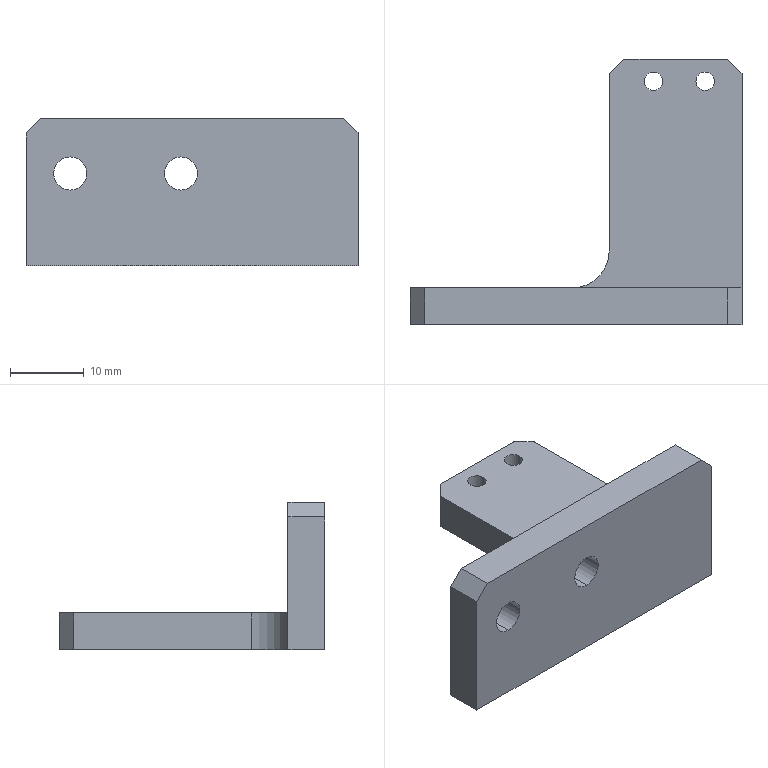Part | STEP file | 10-10 sensor fixing block | 1 solid | 22 faces | box 45 x 36 x 20 mm | volume 7069 mm3 | plane 13 | cylinder 9 | commonest cylinder face diameters 2.5 x4 4.5 x4 10 x1
STEP:
#1=CARTESIAN_POINT('',(34.25,33.,5.));
#2=VERTEX_POINT('',#1);
#3=CARTESIAN_POINT('',(31.75,33.,5.));
#4=VERTEX_POINT('',#3);
#5=CARTESIAN_POINT('',(33.,33.,5.));
#6=DIRECTION('',(0.,0.,-1.));
#7=DIRECTION('',(0.,1.,0.));
#8=AXIS2_PLACEMENT_3D('',#5,#6,#7);
#9=CIRCLE('',#8,1.25);
#10=EDGE_CURVE('',#2,#4,#9,.T.);
#11=ORIENTED_EDGE('',*,*,#10,.F.);
#12=CARTESIAN_POINT('',(34.25,33.,0.));
#13=VERTEX_POINT('',#12);
#14=CARTESIAN_POINT('',(34.25,33.,0.));
#15=DIRECTION('',(0.,0.,-1.));
#16=VECTOR('',#15,1000.);
#17=LINE('',#14,#16);
#18=EDGE_CURVE('',#2,#13,#17,.T.);
#19=ORIENTED_EDGE('',*,*,#18,.T.);
#20=CARTESIAN_POINT('',(31.75,33.,0.));
#21=VERTEX_POINT('',#20);
#22=CARTESIAN_POINT('',(33.,33.,0.));
#23=DIRECTION('',(0.,0.,-1.));
#24=DIRECTION('',(-1.,0.,0.));
#25=AXIS2_PLACEMENT_3D('',#22,#23,#24);
#26=CIRCLE('',#25,1.25);
#27=EDGE_CURVE('',#13,#21,#26,.T.);
#28=ORIENTED_EDGE('',*,*,#27,.T.);
#29=CARTESIAN_POINT('',(31.75,33.,0.));
#30=DIRECTION('',(0.,0.,-1.));
#31=VECTOR('',#30,1000.);
#32=LINE('',#29,#31);
#33=EDGE_CURVE('',#4,#21,#32,.T.);
#34=ORIENTED_EDGE('',*,*,#33,.F.);
#35=EDGE_LOOP('',(#11,#19,#28,#34));
#36=FACE_OUTER_BOUND('',#35,.T.);
#37=CARTESIAN_POINT('',(33.,33.,0.));
#38=DIRECTION('',(0.,0.,-1.));
#39=DIRECTION('',(-1.,0.,0.));
#40=AXIS2_PLACEMENT_3D('',#37,#38,#39);
#41=CYLINDRICAL_SURFACE('',#40,1.25);
#42=ADVANCED_FACE('',(#36),#41,.F.);
#43=CARTESIAN_POINT('',(41.25,33.,5.));
#44=VERTEX_POINT('',#43);
#45=CARTESIAN_POINT('',(38.75,33.,5.));
#46=VERTEX_POINT('',#45);
#47=CARTESIAN_POINT('',(40.,33.,5.));
#48=DIRECTION('',(0.,0.,-1.));
#49=DIRECTION('',(0.,1.,0.));
#50=AXIS2_PLACEMENT_3D('',#47,#48,#49);
#51=CIRCLE('',#50,1.25);
#52=EDGE_CURVE('',#44,#46,#51,.T.);
#53=ORIENTED_EDGE('',*,*,#52,.F.);
#54=CARTESIAN_POINT('',(41.25,33.,0.));
#55=VERTEX_POINT('',#54);
#56=CARTESIAN_POINT('',(41.25,33.,0.));
#57=DIRECTION('',(0.,0.,-1.));
#58=VECTOR('',#57,1000.);
#59=LINE('',#56,#58);
#60=EDGE_CURVE('',#44,#55,#59,.T.);
#61=ORIENTED_EDGE('',*,*,#60,.T.);
#62=CARTESIAN_POINT('',(38.75,33.,0.));
#63=VERTEX_POINT('',#62);
#64=CARTESIAN_POINT('',(40.,33.,0.));
#65=DIRECTION('',(0.,0.,-1.));
#66=DIRECTION('',(-1.,0.,0.));
#67=AXIS2_PLACEMENT_3D('',#64,#65,#66);
#68=CIRCLE('',#67,1.25);
#69=EDGE_CURVE('',#55,#63,#68,.T.);
#70=ORIENTED_EDGE('',*,*,#69,.T.);
#71=CARTESIAN_POINT('',(38.75,33.,0.));
#72=DIRECTION('',(0.,0.,-1.));
#73=VECTOR('',#72,1000.);
#74=LINE('',#71,#73);
#75=EDGE_CURVE('',#46,#63,#74,.T.);
#76=ORIENTED_EDGE('',*,*,#75,.F.);
#77=EDGE_LOOP('',(#53,#61,#70,#76));
#78=FACE_OUTER_BOUND('',#77,.T.);
#79=CARTESIAN_POINT('',(40.,33.,0.));
#80=DIRECTION('',(0.,0.,-1.));
#81=DIRECTION('',(-1.,0.,0.));
#82=AXIS2_PLACEMENT_3D('',#79,#80,#81);
#83=CYLINDRICAL_SURFACE('',#82,1.25);
#84=ADVANCED_FACE('',(#78),#83,.F.);
#85=CARTESIAN_POINT('',(6.,0.,10.25));
#86=VERTEX_POINT('',#85);
#87=CARTESIAN_POINT('',(6.,0.,14.75));
#88=VERTEX_POINT('',#87);
#89=CARTESIAN_POINT('',(6.,0.,12.5));
#90=DIRECTION('',(0.,1.,0.));
#91=DIRECTION('',(0.,0.,1.));
#92=AXIS2_PLACEMENT_3D('',#89,#90,#91);
#93=CIRCLE('',#92,2.25);
#94=EDGE_CURVE('',#86,#88,#93,.T.);
#95=ORIENTED_EDGE('',*,*,#94,.F.);
#96=CARTESIAN_POINT('',(6.,5.,10.25));
#97=VERTEX_POINT('',#96);
#98=CARTESIAN_POINT('',(6.,0.,10.25));
#99=DIRECTION('',(0.,1.,0.));
#100=VECTOR('',#99,1000.);
#101=LINE('',#98,#100);
#102=EDGE_CURVE('',#86,#97,#101,.T.);
#103=ORIENTED_EDGE('',*,*,#102,.T.);
#104=CARTESIAN_POINT('',(6.,5.,14.75));
#105=VERTEX_POINT('',#104);
#106=CARTESIAN_POINT('',(6.,5.,12.5));
#107=DIRECTION('',(0.,1.,0.));
#108=DIRECTION('',(0.,0.,1.));
#109=AXIS2_PLACEMENT_3D('',#106,#107,#108);
#110=CIRCLE('',#109,2.25);
#111=EDGE_CURVE('',#97,#105,#110,.T.);
#112=ORIENTED_EDGE('',*,*,#111,.T.);
#113=CARTESIAN_POINT('',(6.,0.,14.75));
#114=DIRECTION('',(0.,1.,0.));
#115=VECTOR('',#114,1000.);
#116=LINE('',#113,#115);
#117=EDGE_CURVE('',#88,#105,#116,.T.);
#118=ORIENTED_EDGE('',*,*,#117,.F.);
#119=EDGE_LOOP('',(#95,#103,#112,#118));
#120=FACE_OUTER_BOUND('',#119,.T.);
#121=CARTESIAN_POINT('',(6.,0.,12.5));
#122=DIRECTION('',(0.,1.,0.));
#123=DIRECTION('',(0.,0.,1.));
#124=AXIS2_PLACEMENT_3D('',#121,#122,#123);
#125=CYLINDRICAL_SURFACE('',#124,2.25);
#126=ADVANCED_FACE('',(#120),#125,.F.);
#127=CARTESIAN_POINT('',(21.,0.,10.25));
#128=VERTEX_POINT('',#127);
#129=CARTESIAN_POINT('',(21.,0.,14.75));
#130=VERTEX_POINT('',#129);
#131=CARTESIAN_POINT('',(21.,0.,12.5));
#132=DIRECTION('',(0.,1.,0.));
#133=DIRECTION('',(0.,0.,1.));
#134=AXIS2_PLACEMENT_3D('',#131,#132,#133);
#135=CIRCLE('',#134,2.25);
#136=EDGE_CURVE('',#128,#130,#135,.T.);
#137=ORIENTED_EDGE('',*,*,#136,.F.);
#138=CARTESIAN_POINT('',(21.,5.,10.25));
#139=VERTEX_POINT('',#138);
#140=CARTESIAN_POINT('',(21.,0.,10.25));
#141=DIRECTION('',(0.,1.,0.));
#142=VECTOR('',#141,1000.);
#143=LINE('',#140,#142);
#144=EDGE_CURVE('',#128,#139,#143,.T.);
#145=ORIENTED_EDGE('',*,*,#144,.T.);
#146=CARTESIAN_POINT('',(21.,5.,14.75));
#147=VERTEX_POINT('',#146);
#148=CARTESIAN_POINT('',(21.,5.,12.5));
#149=DIRECTION('',(0.,1.,0.));
#150=DIRECTION('',(0.,0.,1.));
#151=AXIS2_PLACEMENT_3D('',#148,#149,#150);
#152=CIRCLE('',#151,2.25);
#153=EDGE_CURVE('',#139,#147,#152,.T.);
#154=ORIENTED_EDGE('',*,*,#153,.T.);
#155=CARTESIAN_POINT('',(21.,0.,14.75));
#156=DIRECTION('',(0.,1.,0.));
#157=VECTOR('',#156,1000.);
#158=LINE('',#155,#157);
#159=EDGE_CURVE('',#130,#147,#158,.T.);
#160=ORIENTED_EDGE('',*,*,#159,.F.);
#161=EDGE_LOOP('',(#137,#145,#154,#160));
#162=FACE_OUTER_BOUND('',#161,.T.);
#163=CARTESIAN_POINT('',(21.,0.,12.5));
#164=DIRECTION('',(0.,1.,0.));
#165=DIRECTION('',(0.,0.,1.));
#166=AXIS2_PLACEMENT_3D('',#163,#164,#165);
#167=CYLINDRICAL_SURFACE('',#166,2.25);
#168=ADVANCED_FACE('',(#162),#167,.F.);
#169=CARTESIAN_POINT('',(6.,0.,12.5));
#170=DIRECTION('',(0.,1.,0.));
#171=DIRECTION('',(0.,0.,1.));
#172=AXIS2_PLACEMENT_3D('',#169,#170,#171);
#173=CIRCLE('',#172,2.25);
#174=EDGE_CURVE('',#88,#86,#173,.T.);
#175=ORIENTED_EDGE('',*,*,#174,.T.);
#176=ORIENTED_EDGE('',*,*,#94,.T.);
#177=EDGE_LOOP('',(#175,#176));
#178=FACE_BOUND('',#177,.T.);
#179=CARTESIAN_POINT('',(21.,0.,12.5));
#180=DIRECTION('',(0.,1.,0.));
#181=DIRECTION('',(0.,0.,1.));
#182=AXIS2_PLACEMENT_3D('',#179,#180,#181);
#183=CIRCLE('',#182,2.25);
#184=EDGE_CURVE('',#130,#128,#183,.T.);
#185=ORIENTED_EDGE('',*,*,#184,.T.);
#186=ORIENTED_EDGE('',*,*,#136,.T.);
#187=EDGE_LOOP('',(#185,#186));
#188=FACE_BOUND('',#187,.T.);
#189=CARTESIAN_POINT('',(45.,0.,18.));
#190=VERTEX_POINT('',#189);
#191=CARTESIAN_POINT('',(45.,0.,0.));
#192=VERTEX_POINT('',#191);
#193=CARTESIAN_POINT('',(45.,0.,20.));
#194=DIRECTION('',(0.,0.,-1.));
#195=VECTOR('',#194,1000.);
#196=LINE('',#193,#195);
#197=EDGE_CURVE('',#190,#192,#196,.T.);
#198=ORIENTED_EDGE('',*,*,#197,.F.);
#199=CARTESIAN_POINT('',(43.,0.,20.));
#200=VERTEX_POINT('',#199);
#201=CARTESIAN_POINT('',(45.,0.,18.));
#202=DIRECTION('',(-0.7071,0.,0.7071));
#203=VECTOR('',#202,1000.);
#204=LINE('',#201,#203);
#205=EDGE_CURVE('',#190,#200,#204,.T.);
#206=ORIENTED_EDGE('',*,*,#205,.T.);
#207=CARTESIAN_POINT('',(2.,0.,20.));
#208=VERTEX_POINT('',#207);
#209=CARTESIAN_POINT('',(45.,0.,20.));
#210=DIRECTION('',(-1.,0.,0.));
#211=VECTOR('',#210,1000.);
#212=LINE('',#209,#211);
#213=EDGE_CURVE('',#200,#208,#212,.T.);
#214=ORIENTED_EDGE('',*,*,#213,.T.);
#215=CARTESIAN_POINT('',(0.,0.,18.));
#216=VERTEX_POINT('',#215);
#217=CARTESIAN_POINT('',(2.,0.,20.));
#218=DIRECTION('',(-0.7071,0.,-0.7071));
#219=VECTOR('',#218,1000.);
#220=LINE('',#217,#219);
#221=EDGE_CURVE('',#208,#216,#220,.T.);
#222=ORIENTED_EDGE('',*,*,#221,.T.);
#223=CARTESIAN_POINT('',(0.,0.,0.));
#224=VERTEX_POINT('',#223);
#225=CARTESIAN_POINT('',(0.,0.,20.));
#226=DIRECTION('',(0.,0.,-1.));
#227=VECTOR('',#226,1000.);
#228=LINE('',#225,#227);
#229=EDGE_CURVE('',#216,#224,#228,.T.);
#230=ORIENTED_EDGE('',*,*,#229,.T.);
#231=CARTESIAN_POINT('',(45.,0.,0.));
#232=DIRECTION('',(-1.,0.,0.));
#233=VECTOR('',#232,1000.);
#234=LINE('',#231,#233);
#235=EDGE_CURVE('',#192,#224,#234,.T.);
#236=ORIENTED_EDGE('',*,*,#235,.F.);
#237=EDGE_LOOP('',(#198,#206,#214,#222,#230,#236));
#238=FACE_OUTER_BOUND('',#237,.T.);
#239=CARTESIAN_POINT('',(45.,0.,20.));
#240=DIRECTION('',(0.,1.,0.));
#241=DIRECTION('',(0.,0.,1.));
#242=AXIS2_PLACEMENT_3D('',#239,#240,#241);
#243=PLANE('',#242);
#244=ADVANCED_FACE('',(#178,#188,#238),#243,.F.);
#245=CARTESIAN_POINT('',(33.,33.,0.));
#246=DIRECTION('',(0.,0.,-1.));
#247=DIRECTION('',(-1.,0.,0.));
#248=AXIS2_PLACEMENT_3D('',#245,#246,#247);
#249=CIRCLE('',#248,1.25);
#250=EDGE_CURVE('',#21,#13,#249,.T.);
#251=ORIENTED_EDGE('',*,*,#250,.F.);
#252=ORIENTED_EDGE('',*,*,#27,.F.);
#253=EDGE_LOOP('',(#251,#252));
#254=FACE_BOUND('',#253,.T.);
#255=CARTESIAN_POINT('',(40.,33.,0.));
#256=DIRECTION('',(0.,0.,-1.));
#257=DIRECTION('',(-1.,0.,0.));
#258=AXIS2_PLACEMENT_3D('',#255,#256,#257);
#259=CIRCLE('',#258,1.25);
#260=EDGE_CURVE('',#63,#55,#259,.T.);
#261=ORIENTED_EDGE('',*,*,#260,.F.);
#262=ORIENTED_EDGE('',*,*,#69,.F.);
#263=EDGE_LOOP('',(#261,#262));
#264=FACE_BOUND('',#263,.T.);
#265=CARTESIAN_POINT('',(27.,34.,0.));
#266=VERTEX_POINT('',#265);
#267=CARTESIAN_POINT('',(27.,10.,0.));
#268=VERTEX_POINT('',#267);
#269=CARTESIAN_POINT('',(27.,5.,0.));
#270=DIRECTION('',(0.,-1.,0.));
#271=VECTOR('',#270,1000.);
#272=LINE('',#269,#271);
#273=EDGE_CURVE('',#266,#268,#272,.T.);
#274=ORIENTED_EDGE('',*,*,#273,.F.);
#275=CARTESIAN_POINT('',(29.,36.,0.));
#276=VERTEX_POINT('',#275);
#277=CARTESIAN_POINT('',(27.,34.,0.));
#278=DIRECTION('',(0.7071,0.7071,0.));
#279=VECTOR('',#278,1000.);
#280=LINE('',#277,#279);
#281=EDGE_CURVE('',#266,#276,#280,.T.);
#282=ORIENTED_EDGE('',*,*,#281,.T.);
#283=CARTESIAN_POINT('',(43.,36.,0.));
#284=VERTEX_POINT('',#283);
#285=CARTESIAN_POINT('',(45.,36.,0.));
#286=DIRECTION('',(-1.,0.,0.));
#287=VECTOR('',#286,1000.);
#288=LINE('',#285,#287);
#289=EDGE_CURVE('',#284,#276,#288,.T.);
#290=ORIENTED_EDGE('',*,*,#289,.F.);
#291=CARTESIAN_POINT('',(45.,34.,0.));
#292=VERTEX_POINT('',#291);
#293=CARTESIAN_POINT('',(45.,34.,0.));
#294=DIRECTION('',(0.7071,-0.7071,0.));
#295=VECTOR('',#294,1000.);
#296=LINE('',#293,#295);
#297=EDGE_CURVE('',#284,#292,#296,.T.);
#298=ORIENTED_EDGE('',*,*,#297,.T.);
#299=CARTESIAN_POINT('',(45.,0.,0.));
#300=DIRECTION('',(0.,1.,0.));
#301=VECTOR('',#300,1000.);
#302=LINE('',#299,#301);
#303=EDGE_CURVE('',#192,#292,#302,.T.);
#304=ORIENTED_EDGE('',*,*,#303,.F.);
#305=ORIENTED_EDGE('',*,*,#235,.T.);
#306=CARTESIAN_POINT('',(0.,5.,0.));
#307=VERTEX_POINT('',#306);
#308=CARTESIAN_POINT('',(0.,0.,0.));
#309=DIRECTION('',(0.,1.,0.));
#310=VECTOR('',#309,1000.);
#311=LINE('',#308,#310);
#312=EDGE_CURVE('',#224,#307,#311,.T.);
#313=ORIENTED_EDGE('',*,*,#312,.T.);
#314=CARTESIAN_POINT('',(22.,5.,0.));
#315=VERTEX_POINT('',#314);
#316=CARTESIAN_POINT('',(0.,5.,0.));
#317=DIRECTION('',(-1.,0.,0.));
#318=VECTOR('',#317,1000.);
#319=LINE('',#316,#318);
#320=EDGE_CURVE('',#315,#307,#319,.T.);
#321=ORIENTED_EDGE('',*,*,#320,.F.);
#322=CARTESIAN_POINT('',(22.,10.,0.));
#323=DIRECTION('',(0.,0.,1.));
#324=DIRECTION('',(1.,0.,0.));
#325=AXIS2_PLACEMENT_3D('',#322,#323,#324);
#326=CIRCLE('',#325,5.);
#327=EDGE_CURVE('',#315,#268,#326,.T.);
#328=ORIENTED_EDGE('',*,*,#327,.T.);
#329=EDGE_LOOP('',(#274,#282,#290,#298,#304,#305,#313,#321,#328));
#330=FACE_OUTER_BOUND('',#329,.T.);
#331=CARTESIAN_POINT('',(45.,0.,0.));
#332=DIRECTION('',(0.,0.,1.));
#333=DIRECTION('',(1.,0.,0.));
#334=AXIS2_PLACEMENT_3D('',#331,#332,#333);
#335=PLANE('',#334);
#336=ADVANCED_FACE('',(#254,#264,#330),#335,.F.);
#337=ORIENTED_EDGE('',*,*,#289,.T.);
#338=CARTESIAN_POINT('',(29.,36.,5.));
#339=VERTEX_POINT('',#338);
#340=CARTESIAN_POINT('',(29.,36.,0.));
#341=DIRECTION('',(0.,0.,1.));
#342=VECTOR('',#341,1000.);
#343=LINE('',#340,#342);
#344=EDGE_CURVE('',#276,#339,#343,.T.);
#345=ORIENTED_EDGE('',*,*,#344,.T.);
#346=CARTESIAN_POINT('',(43.,36.,5.));
#347=VERTEX_POINT('',#346);
#348=CARTESIAN_POINT('',(45.,36.,5.));
#349=DIRECTION('',(-1.,0.,0.));
#350=VECTOR('',#349,1000.);
#351=LINE('',#348,#350);
#352=EDGE_CURVE('',#347,#339,#351,.T.);
#353=ORIENTED_EDGE('',*,*,#352,.F.);
#354=CARTESIAN_POINT('',(43.,36.,0.));
#355=DIRECTION('',(0.,0.,-1.));
#356=VECTOR('',#355,1000.);
#357=LINE('',#354,#356);
#358=EDGE_CURVE('',#347,#284,#357,.T.);
#359=ORIENTED_EDGE('',*,*,#358,.T.);
#360=EDGE_LOOP('',(#337,#345,#353,#359));
#361=FACE_OUTER_BOUND('',#360,.T.);
#362=CARTESIAN_POINT('',(45.,36.,0.));
#363=DIRECTION('',(0.,-1.,0.));
#364=DIRECTION('',(0.,0.,-1.));
#365=AXIS2_PLACEMENT_3D('',#362,#363,#364);
#366=PLANE('',#365);
#367=ADVANCED_FACE('',(#361),#366,.F.);
#368=CARTESIAN_POINT('',(33.,33.,5.));
#369=DIRECTION('',(0.,0.,-1.));
#370=DIRECTION('',(0.,1.,0.));
#371=AXIS2_PLACEMENT_3D('',#368,#369,#370);
#372=CIRCLE('',#371,1.25);
#373=EDGE_CURVE('',#4,#2,#372,.T.);
#374=ORIENTED_EDGE('',*,*,#373,.T.);
#375=ORIENTED_EDGE('',*,*,#10,.T.);
#376=EDGE_LOOP('',(#374,#375));
#377=FACE_BOUND('',#376,.T.);
#378=CARTESIAN_POINT('',(40.,33.,5.));
#379=DIRECTION('',(0.,0.,-1.));
#380=DIRECTION('',(0.,1.,0.));
#381=AXIS2_PLACEMENT_3D('',#378,#379,#380);
#382=CIRCLE('',#381,1.25);
#383=EDGE_CURVE('',#46,#44,#382,.T.);
#384=ORIENTED_EDGE('',*,*,#383,.T.);
#385=ORIENTED_EDGE('',*,*,#52,.T.);
#386=EDGE_LOOP('',(#384,#385));
#387=FACE_BOUND('',#386,.T.);
#388=ORIENTED_EDGE('',*,*,#352,.T.);
#389=CARTESIAN_POINT('',(27.,34.,5.));
#390=VERTEX_POINT('',#389);
#391=CARTESIAN_POINT('',(27.,34.,5.));
#392=DIRECTION('',(-0.7071,-0.7071,0.));
#393=VECTOR('',#392,1000.);
#394=LINE('',#391,#393);
#395=EDGE_CURVE('',#339,#390,#394,.T.);
#396=ORIENTED_EDGE('',*,*,#395,.T.);
#397=CARTESIAN_POINT('',(27.,10.,5.));
#398=VERTEX_POINT('',#397);
#399=CARTESIAN_POINT('',(27.,36.,5.));
#400=DIRECTION('',(0.,-1.,0.));
#401=VECTOR('',#400,1000.);
#402=LINE('',#399,#401);
#403=EDGE_CURVE('',#390,#398,#402,.T.);
#404=ORIENTED_EDGE('',*,*,#403,.T.);
#405=CARTESIAN_POINT('',(22.,5.,5.));
#406=VERTEX_POINT('',#405);
#407=CARTESIAN_POINT('',(22.,10.,5.));
#408=DIRECTION('',(0.,0.,-1.));
#409=DIRECTION('',(0.,1.,0.));
#410=AXIS2_PLACEMENT_3D('',#407,#408,#409);
#411=CIRCLE('',#410,5.);
#412=EDGE_CURVE('',#398,#406,#411,.T.);
#413=ORIENTED_EDGE('',*,*,#412,.T.);
#414=CARTESIAN_POINT('',(45.,5.,5.));
#415=VERTEX_POINT('',#414);
#416=CARTESIAN_POINT('',(45.,5.,5.));
#417=DIRECTION('',(-1.,0.,0.));
#418=VECTOR('',#417,1000.);
#419=LINE('',#416,#418);
#420=EDGE_CURVE('',#415,#406,#419,.T.);
#421=ORIENTED_EDGE('',*,*,#420,.F.);
#422=CARTESIAN_POINT('',(45.,34.,5.));
#423=VERTEX_POINT('',#422);
#424=CARTESIAN_POINT('',(45.,36.,5.));
#425=DIRECTION('',(0.,-1.,0.));
#426=VECTOR('',#425,1000.);
#427=LINE('',#424,#426);
#428=EDGE_CURVE('',#423,#415,#427,.T.);
#429=ORIENTED_EDGE('',*,*,#428,.F.);
#430=CARTESIAN_POINT('',(45.,34.,5.));
#431=DIRECTION('',(-0.7071,0.7071,0.));
#432=VECTOR('',#431,1000.);
#433=LINE('',#430,#432);
#434=EDGE_CURVE('',#423,#347,#433,.T.);
#435=ORIENTED_EDGE('',*,*,#434,.T.);
#436=EDGE_LOOP('',(#388,#396,#404,#413,#421,#429,#435));
#437=FACE_OUTER_BOUND('',#436,.T.);
#438=CARTESIAN_POINT('',(45.,36.,5.));
#439=DIRECTION('',(0.,0.,-1.));
#440=DIRECTION('',(0.,1.,0.));
#441=AXIS2_PLACEMENT_3D('',#438,#439,#440);
#442=PLANE('',#441);
#443=ADVANCED_FACE('',(#377,#387,#437),#442,.F.);
#444=CARTESIAN_POINT('',(6.,5.,12.5));
#445=DIRECTION('',(0.,1.,0.));
#446=DIRECTION('',(0.,0.,1.));
#447=AXIS2_PLACEMENT_3D('',#444,#445,#446);
#448=CIRCLE('',#447,2.25);
#449=EDGE_CURVE('',#105,#97,#448,.T.);
#450=ORIENTED_EDGE('',*,*,#449,.F.);
#451=ORIENTED_EDGE('',*,*,#111,.F.);
#452=EDGE_LOOP('',(#450,#451));
#453=FACE_BOUND('',#452,.T.);
#454=CARTESIAN_POINT('',(21.,5.,12.5));
#455=DIRECTION('',(0.,1.,0.));
#456=DIRECTION('',(0.,0.,1.));
#457=AXIS2_PLACEMENT_3D('',#454,#455,#456);
#458=CIRCLE('',#457,2.25);
#459=EDGE_CURVE('',#147,#139,#458,.T.);
#460=ORIENTED_EDGE('',*,*,#459,.F.);
#461=ORIENTED_EDGE('',*,*,#153,.F.);
#462=EDGE_LOOP('',(#460,#461));
#463=FACE_BOUND('',#462,.T.);
#464=ORIENTED_EDGE('',*,*,#420,.T.);
#465=CARTESIAN_POINT('',(22.,5.,0.));
#466=DIRECTION('',(0.,0.,-1.));
#467=VECTOR('',#466,1000.);
#468=LINE('',#465,#467);
#469=EDGE_CURVE('',#406,#315,#468,.T.);
#470=ORIENTED_EDGE('',*,*,#469,.T.);
#471=ORIENTED_EDGE('',*,*,#320,.T.);
#472=CARTESIAN_POINT('',(0.,5.,18.));
#473=VERTEX_POINT('',#472);
#474=CARTESIAN_POINT('',(0.,5.,5.));
#475=DIRECTION('',(0.,0.,1.));
#476=VECTOR('',#475,1000.);
#477=LINE('',#474,#476);
#478=EDGE_CURVE('',#307,#473,#477,.T.);
#479=ORIENTED_EDGE('',*,*,#478,.T.);
#480=CARTESIAN_POINT('',(2.,5.,20.));
#481=VERTEX_POINT('',#480);
#482=CARTESIAN_POINT('',(2.,5.,20.));
#483=DIRECTION('',(0.7071,0.,0.7071));
#484=VECTOR('',#483,1000.);
#485=LINE('',#482,#484);
#486=EDGE_CURVE('',#473,#481,#485,.T.);
#487=ORIENTED_EDGE('',*,*,#486,.T.);
#488=CARTESIAN_POINT('',(43.,5.,20.));
#489=VERTEX_POINT('',#488);
#490=CARTESIAN_POINT('',(45.,5.,20.));
#491=DIRECTION('',(-1.,0.,0.));
#492=VECTOR('',#491,1000.);
#493=LINE('',#490,#492);
#494=EDGE_CURVE('',#489,#481,#493,.T.);
#495=ORIENTED_EDGE('',*,*,#494,.F.);
#496=CARTESIAN_POINT('',(45.,5.,18.));
#497=VERTEX_POINT('',#496);
#498=CARTESIAN_POINT('',(45.,5.,18.));
#499=DIRECTION('',(0.7071,0.,-0.7071));
#500=VECTOR('',#499,1000.);
#501=LINE('',#498,#500);
#502=EDGE_CURVE('',#489,#497,#501,.T.);
#503=ORIENTED_EDGE('',*,*,#502,.T.);
#504=CARTESIAN_POINT('',(45.,5.,5.));
#505=DIRECTION('',(0.,0.,1.));
#506=VECTOR('',#505,1000.);
#507=LINE('',#504,#506);
#508=EDGE_CURVE('',#415,#497,#507,.T.);
#509=ORIENTED_EDGE('',*,*,#508,.F.);
#510=EDGE_LOOP('',(#464,#470,#471,#479,#487,#495,#503,#509));
#511=FACE_OUTER_BOUND('',#510,.T.);
#512=CARTESIAN_POINT('',(45.,5.,5.));
#513=DIRECTION('',(0.,-1.,0.));
#514=DIRECTION('',(0.,0.,-1.));
#515=AXIS2_PLACEMENT_3D('',#512,#513,#514);
#516=PLANE('',#515);
#517=ADVANCED_FACE('',(#453,#463,#511),#516,.F.);
#518=ORIENTED_EDGE('',*,*,#213,.F.);
#519=CARTESIAN_POINT('',(43.,5.,20.));
#520=DIRECTION('',(0.,1.,0.));
#521=VECTOR('',#520,1000.);
#522=LINE('',#519,#521);
#523=EDGE_CURVE('',#200,#489,#522,.T.);
#524=ORIENTED_EDGE('',*,*,#523,.T.);
#525=ORIENTED_EDGE('',*,*,#494,.T.);
#526=CARTESIAN_POINT('',(2.,5.,20.));
#527=DIRECTION('',(0.,-1.,0.));
#528=VECTOR('',#527,1000.);
#529=LINE('',#526,#528);
#530=EDGE_CURVE('',#481,#208,#529,.T.);
#531=ORIENTED_EDGE('',*,*,#530,.T.);
#532=EDGE_LOOP('',(#518,#524,#525,#531));
#533=FACE_OUTER_BOUND('',#532,.T.);
#534=CARTESIAN_POINT('',(45.,5.,20.));
#535=DIRECTION('',(0.,0.,-1.));
#536=DIRECTION('',(-1.,0.,0.));
#537=AXIS2_PLACEMENT_3D('',#534,#535,#536);
#538=PLANE('',#537);
#539=ADVANCED_FACE('',(#533),#538,.F.);
#540=ORIENTED_EDGE('',*,*,#303,.T.);
#541=CARTESIAN_POINT('',(45.,34.,5.));
#542=DIRECTION('',(0.,0.,1.));
#543=VECTOR('',#542,1000.);
#544=LINE('',#541,#543);
#545=EDGE_CURVE('',#292,#423,#544,.T.);
#546=ORIENTED_EDGE('',*,*,#545,.T.);
#547=ORIENTED_EDGE('',*,*,#428,.T.);
#548=ORIENTED_EDGE('',*,*,#508,.T.);
#549=CARTESIAN_POINT('',(45.,0.,18.));
#550=DIRECTION('',(0.,-1.,0.));
#551=VECTOR('',#550,1000.);
#552=LINE('',#549,#551);
#553=EDGE_CURVE('',#497,#190,#552,.T.);
#554=ORIENTED_EDGE('',*,*,#553,.T.);
#555=ORIENTED_EDGE('',*,*,#197,.T.);
#556=EDGE_LOOP('',(#540,#546,#547,#548,#554,#555));
#557=FACE_OUTER_BOUND('',#556,.T.);
#558=CARTESIAN_POINT('',(45.,0.,0.));
#559=DIRECTION('',(1.,0.,0.));
#560=DIRECTION('',(0.,0.,-1.));
#561=AXIS2_PLACEMENT_3D('',#558,#559,#560);
#562=PLANE('',#561);
#563=ADVANCED_FACE('',(#557),#562,.T.);
#564=ORIENTED_EDGE('',*,*,#478,.F.);
#565=ORIENTED_EDGE('',*,*,#312,.F.);
#566=ORIENTED_EDGE('',*,*,#229,.F.);
#567=CARTESIAN_POINT('',(0.,0.,18.));
#568=DIRECTION('',(0.,1.,0.));
#569=VECTOR('',#568,1000.);
#570=LINE('',#567,#569);
#571=EDGE_CURVE('',#216,#473,#570,.T.);
#572=ORIENTED_EDGE('',*,*,#571,.T.);
#573=EDGE_LOOP('',(#564,#565,#566,#572));
#574=FACE_OUTER_BOUND('',#573,.T.);
#575=CARTESIAN_POINT('',(0.,0.,0.));
#576=DIRECTION('',(1.,0.,0.));
#577=DIRECTION('',(0.,0.,-1.));
#578=AXIS2_PLACEMENT_3D('',#575,#576,#577);
#579=PLANE('',#578);
#580=ADVANCED_FACE('',(#574),#579,.F.);
#581=ORIENTED_EDGE('',*,*,#297,.F.);
#582=ORIENTED_EDGE('',*,*,#358,.F.);
#583=ORIENTED_EDGE('',*,*,#434,.F.);
#584=ORIENTED_EDGE('',*,*,#545,.F.);
#585=EDGE_LOOP('',(#581,#582,#583,#584));
#586=FACE_OUTER_BOUND('',#585,.T.);
#587=CARTESIAN_POINT('',(45.,34.,0.));
#588=DIRECTION('',(0.7071,0.7071,0.));
#589=DIRECTION('',(-0.7071,0.7071,0.));
#590=AXIS2_PLACEMENT_3D('',#587,#588,#589);
#591=PLANE('',#590);
#592=ADVANCED_FACE('',(#586),#591,.T.);
#593=ORIENTED_EDGE('',*,*,#502,.F.);
#594=ORIENTED_EDGE('',*,*,#523,.F.);
#595=ORIENTED_EDGE('',*,*,#205,.F.);
#596=ORIENTED_EDGE('',*,*,#553,.F.);
#597=EDGE_LOOP('',(#593,#594,#595,#596));
#598=FACE_OUTER_BOUND('',#597,.T.);
#599=CARTESIAN_POINT('',(45.,0.,18.));
#600=DIRECTION('',(0.7071,0.,0.7071));
#601=DIRECTION('',(0.7071,0.,-0.7071));
#602=AXIS2_PLACEMENT_3D('',#599,#600,#601);
#603=PLANE('',#602);
#604=ADVANCED_FACE('',(#598),#603,.T.);
#605=ORIENTED_EDGE('',*,*,#486,.F.);
#606=ORIENTED_EDGE('',*,*,#571,.F.);
#607=ORIENTED_EDGE('',*,*,#221,.F.);
#608=ORIENTED_EDGE('',*,*,#530,.F.);
#609=EDGE_LOOP('',(#605,#606,#607,#608));
#610=FACE_OUTER_BOUND('',#609,.T.);
#611=CARTESIAN_POINT('',(2.,5.,20.));
#612=DIRECTION('',(0.7071,0.,-0.7071));
#613=DIRECTION('',(-0.7071,0.,-0.7071));
#614=AXIS2_PLACEMENT_3D('',#611,#612,#613);
#615=PLANE('',#614);
#616=ADVANCED_FACE('',(#610),#615,.F.);
#617=ORIENTED_EDGE('',*,*,#144,.F.);
#618=ORIENTED_EDGE('',*,*,#184,.F.);
#619=ORIENTED_EDGE('',*,*,#159,.T.);
#620=ORIENTED_EDGE('',*,*,#459,.T.);
#621=EDGE_LOOP('',(#617,#618,#619,#620));
#622=FACE_OUTER_BOUND('',#621,.T.);
#623=CARTESIAN_POINT('',(21.,0.,12.5));
#624=DIRECTION('',(0.,1.,0.));
#625=DIRECTION('',(0.,0.,1.));
#626=AXIS2_PLACEMENT_3D('',#623,#624,#625);
#627=CYLINDRICAL_SURFACE('',#626,2.25);
#628=ADVANCED_FACE('',(#622),#627,.F.);
#629=ORIENTED_EDGE('',*,*,#102,.F.);
#630=ORIENTED_EDGE('',*,*,#174,.F.);
#631=ORIENTED_EDGE('',*,*,#117,.T.);
#632=ORIENTED_EDGE('',*,*,#449,.T.);
#633=EDGE_LOOP('',(#629,#630,#631,#632));
#634=FACE_OUTER_BOUND('',#633,.T.);
#635=CARTESIAN_POINT('',(6.,0.,12.5));
#636=DIRECTION('',(0.,1.,0.));
#637=DIRECTION('',(0.,0.,1.));
#638=AXIS2_PLACEMENT_3D('',#635,#636,#637);
#639=CYLINDRICAL_SURFACE('',#638,2.25);
#640=ADVANCED_FACE('',(#634),#639,.F.);
#641=ORIENTED_EDGE('',*,*,#60,.F.);
#642=ORIENTED_EDGE('',*,*,#383,.F.);
#643=ORIENTED_EDGE('',*,*,#75,.T.);
#644=ORIENTED_EDGE('',*,*,#260,.T.);
#645=EDGE_LOOP('',(#641,#642,#643,#644));
#646=FACE_OUTER_BOUND('',#645,.T.);
#647=CARTESIAN_POINT('',(40.,33.,0.));
#648=DIRECTION('',(0.,0.,-1.));
#649=DIRECTION('',(-1.,0.,0.));
#650=AXIS2_PLACEMENT_3D('',#647,#648,#649);
#651=CYLINDRICAL_SURFACE('',#650,1.25);
#652=ADVANCED_FACE('',(#646),#651,.F.);
#653=ORIENTED_EDGE('',*,*,#18,.F.);
#654=ORIENTED_EDGE('',*,*,#373,.F.);
#655=ORIENTED_EDGE('',*,*,#33,.T.);
#656=ORIENTED_EDGE('',*,*,#250,.T.);
#657=EDGE_LOOP('',(#653,#654,#655,#656));
#658=FACE_OUTER_BOUND('',#657,.T.);
#659=CARTESIAN_POINT('',(33.,33.,0.));
#660=DIRECTION('',(0.,0.,-1.));
#661=DIRECTION('',(-1.,0.,0.));
#662=AXIS2_PLACEMENT_3D('',#659,#660,#661);
#663=CYLINDRICAL_SURFACE('',#662,1.25);
#664=ADVANCED_FACE('',(#658),#663,.F.);
#665=ORIENTED_EDGE('',*,*,#403,.F.);
#666=CARTESIAN_POINT('',(27.,34.,10.));
#667=DIRECTION('',(0.,0.,-1.));
#668=VECTOR('',#667,1000.);
#669=LINE('',#666,#668);
#670=EDGE_CURVE('',#390,#266,#669,.T.);
#671=ORIENTED_EDGE('',*,*,#670,.T.);
#672=ORIENTED_EDGE('',*,*,#273,.T.);
#673=CARTESIAN_POINT('',(27.,10.,5.));
#674=DIRECTION('',(0.,0.,1.));
#675=VECTOR('',#674,1000.);
#676=LINE('',#673,#675);
#677=EDGE_CURVE('',#268,#398,#676,.T.);
#678=ORIENTED_EDGE('',*,*,#677,.T.);
#679=EDGE_LOOP('',(#665,#671,#672,#678));
#680=FACE_OUTER_BOUND('',#679,.T.);
#681=CARTESIAN_POINT('',(27.,5.,10.));
#682=DIRECTION('',(1.,0.,0.));
#683=DIRECTION('',(0.,0.,-1.));
#684=AXIS2_PLACEMENT_3D('',#681,#682,#683);
#685=PLANE('',#684);
#686=ADVANCED_FACE('',(#680),#685,.F.);
#687=ORIENTED_EDGE('',*,*,#412,.F.);
#688=ORIENTED_EDGE('',*,*,#677,.F.);
#689=ORIENTED_EDGE('',*,*,#327,.F.);
#690=ORIENTED_EDGE('',*,*,#469,.F.);
#691=EDGE_LOOP('',(#687,#688,#689,#690));
#692=FACE_OUTER_BOUND('',#691,.T.);
#693=CARTESIAN_POINT('',(22.,10.,5.));
#694=DIRECTION('',(0.,0.,1.));
#695=DIRECTION('',(0.,-1.,0.));
#696=AXIS2_PLACEMENT_3D('',#693,#694,#695);
#697=CYLINDRICAL_SURFACE('',#696,5.);
#698=ADVANCED_FACE('',(#692),#697,.F.);
#699=ORIENTED_EDGE('',*,*,#395,.F.);
#700=ORIENTED_EDGE('',*,*,#344,.F.);
#701=ORIENTED_EDGE('',*,*,#281,.F.);
#702=ORIENTED_EDGE('',*,*,#670,.F.);
#703=EDGE_LOOP('',(#699,#700,#701,#702));
#704=FACE_OUTER_BOUND('',#703,.T.);
#705=CARTESIAN_POINT('',(27.,34.,10.));
#706=DIRECTION('',(0.7071,-0.7071,0.));
#707=DIRECTION('',(0.7071,0.7071,0.));
#708=AXIS2_PLACEMENT_3D('',#705,#706,#707);
#709=PLANE('',#708);
#710=ADVANCED_FACE('',(#704),#709,.F.);
#711=CLOSED_SHELL('',(#42,#84,#126,#168,#244,#336,#367,#443,#517,#539,#563,#580,#592,#604,#616,#628,#640,#652,#664,#686,#698,#710));
#712=MANIFOLD_SOLID_BREP('',#711);
#713=CARTESIAN_POINT('',(0.,0.,0.));
#714=DIRECTION('',(0.,0.,1.));
#715=DIRECTION('',(1.,0.,0.));
#716=AXIS2_PLACEMENT_3D('',#713,#714,#715);
#717=(LENGTH_UNIT()NAMED_UNIT(*)SI_UNIT(.MILLI.,.METRE.));
#718=UNCERTAINTY_MEASURE_WITH_UNIT(LENGTH_MEASURE(0.00001),#717,'','');
#719=(NAMED_UNIT(*)PLANE_ANGLE_UNIT()SI_UNIT($,.RADIAN.));
#720=(NAMED_UNIT(*)SI_UNIT($,.STERADIAN.)SOLID_ANGLE_UNIT());
#721=(GEOMETRIC_REPRESENTATION_CONTEXT(3)GLOBAL_UNCERTAINTY_ASSIGNED_CONTEXT((#718))GLOBAL_UNIT_ASSIGNED_CONTEXT((#717,#719,#720))REPRESENTATION_CONTEXT('',''));
#722=ADVANCED_BREP_SHAPE_REPRESENTATION('',(#712,#716),#721);